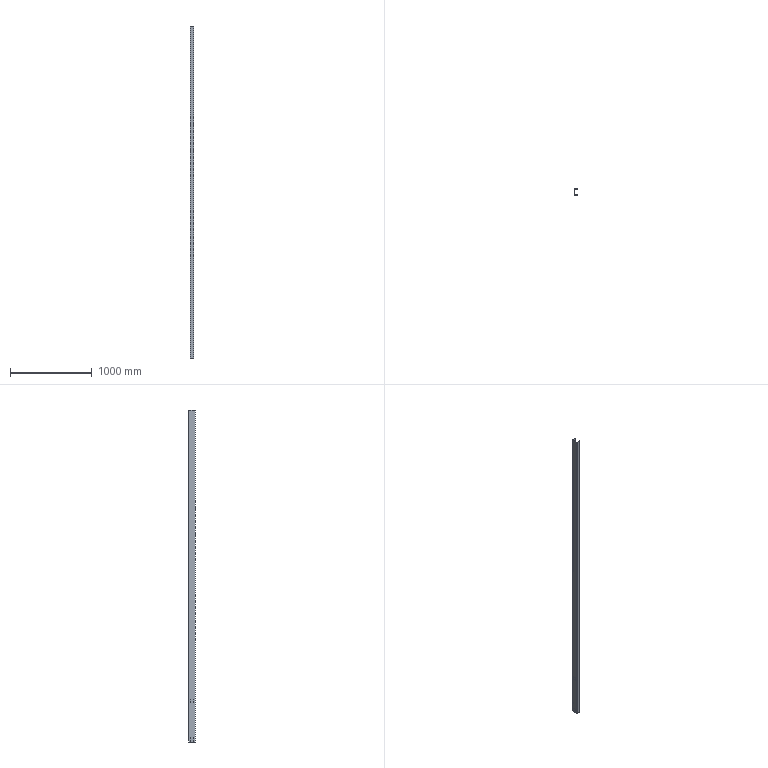Part | STEP file | BCC3 H12_7B | 1 solid | 42 faces | box 40 x 75 x 4068 mm | volume 2791952 mm3 | cylinder 28 | plane 14 | commonest cylinder face diameters 10 x16 12 x12